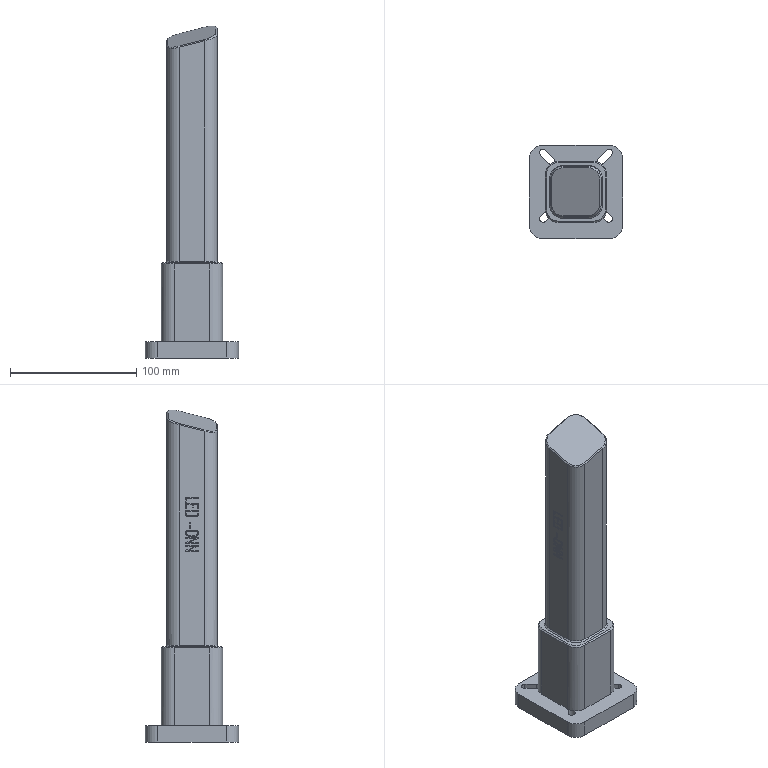Part | NX | features solid 2 | 1 solid | 158 faces | box 74 x 74 x 263.009 mm | volume 474904 mm3 | plane 103 | cylinder 34 | spline 13 | cone 8 | commonest cylinder face diameters 5.5 x20 20 x12 10 x2